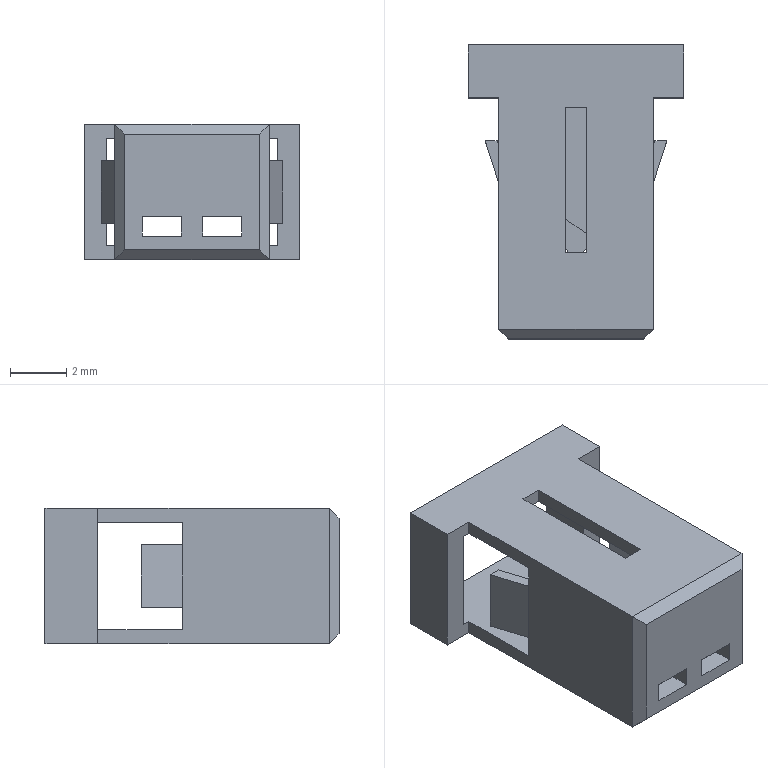Part | SolidWorks | features ICE 9, Chamfer 1, Draft 1, Extrusion 1, Scale 1 | 1 solid | 61 faces | box 7.7 x 10.5 x 4.83 mm | volume 101.737 mm3 | plane 59 | cone 2